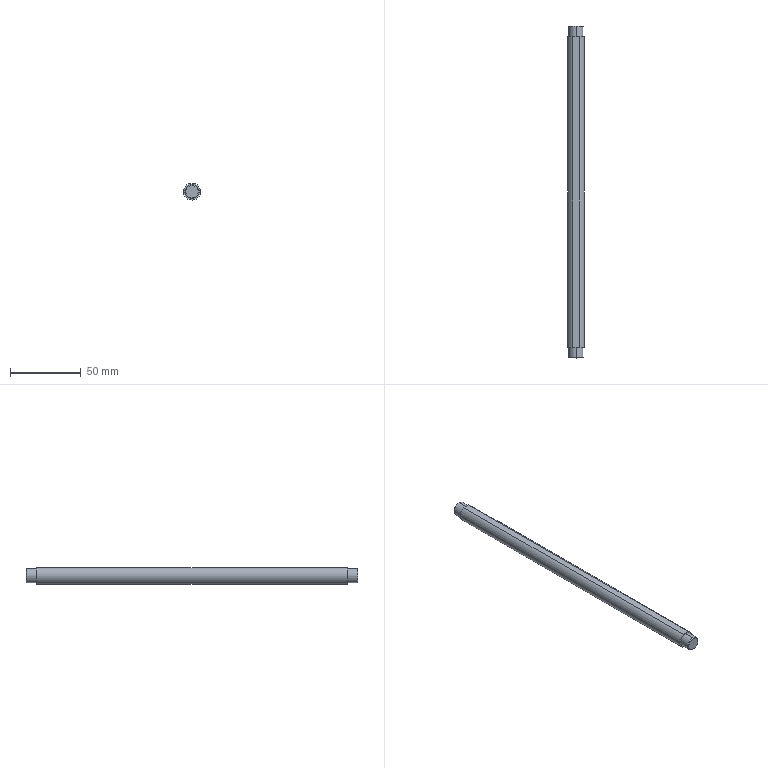Part | NX | features BREP 1 | 1 solid | 15 faces | box 12 x 235.2 x 11.5 mm | volume 25713 mm3 | cylinder 6 | plane 5 | cone 4 | commonest cylinder face diameters 10 x4 12 x2
STEP:
#1=CARTESIAN_POINT('',(0.,-117.1,-5.));
#2=VERTEX_POINT('',#1);
#3=CARTESIAN_POINT('',(0.,-117.6,-4.5));
#4=VERTEX_POINT('',#3);
#5=CARTESIAN_POINT('',(0.,-117.6,-4.5));
#6=DIRECTION('',(0.,0.7071,-0.7071));
#7=VECTOR('',#6,1000.);
#8=LINE('',#5,#7);
#9=EDGE_CURVE('',#2,#4,#8,.F.);
#10=ORIENTED_EDGE('',*,*,#9,.T.);
#11=CARTESIAN_POINT('',(0.,-117.6,4.5));
#12=VERTEX_POINT('',#11);
#13=CARTESIAN_POINT('',(0.,-117.6,0.));
#14=DIRECTION('',(0.,-1.,0.));
#15=DIRECTION('',(0.,0.,1.));
#16=AXIS2_PLACEMENT_3D('',#13,#14,#15);
#17=CIRCLE('',#16,4.5);
#18=EDGE_CURVE('',#12,#4,#17,.T.);
#19=ORIENTED_EDGE('',*,*,#18,.F.);
#20=CARTESIAN_POINT('',(0.,-117.1,5.));
#21=VERTEX_POINT('',#20);
#22=CARTESIAN_POINT('',(0.,-117.6,4.5));
#23=DIRECTION('',(0.,0.7071,0.7071));
#24=VECTOR('',#23,1000.);
#25=LINE('',#22,#24);
#26=EDGE_CURVE('',#21,#12,#25,.F.);
#27=ORIENTED_EDGE('',*,*,#26,.F.);
#28=CARTESIAN_POINT('',(0.,-117.1,0.));
#29=DIRECTION('',(0.,1.,0.));
#30=DIRECTION('',(0.,0.,1.));
#31=AXIS2_PLACEMENT_3D('',#28,#29,#30);
#32=CIRCLE('',#31,5.);
#33=EDGE_CURVE('',#2,#21,#32,.T.);
#34=ORIENTED_EDGE('',*,*,#33,.F.);
#35=EDGE_LOOP('',(#10,#19,#27,#34));
#36=FACE_BOUND('',#35,.T.);
#37=CARTESIAN_POINT('',(0.,-117.6,0.));
#38=DIRECTION('',(0.,1.,0.));
#39=DIRECTION('',(0.,0.,1.));
#40=AXIS2_PLACEMENT_3D('',#37,#38,#39);
#41=CONICAL_SURFACE('',#40,4.5,0.7854);
#42=ADVANCED_FACE('',(#36),#41,.T.);
#43=CARTESIAN_POINT('',(0.,117.6,4.5));
#44=VERTEX_POINT('',#43);
#45=CARTESIAN_POINT('',(0.,117.1,5.));
#46=VERTEX_POINT('',#45);
#47=CARTESIAN_POINT('',(0.,117.1,5.));
#48=DIRECTION('',(0.,-0.7071,0.7071));
#49=VECTOR('',#48,1000.);
#50=LINE('',#47,#49);
#51=EDGE_CURVE('',#44,#46,#50,.T.);
#52=ORIENTED_EDGE('',*,*,#51,.F.);
#53=CARTESIAN_POINT('',(0.,117.6,-4.5));
#54=VERTEX_POINT('',#53);
#55=CARTESIAN_POINT('',(0.,117.6,0.));
#56=DIRECTION('',(0.,1.,0.));
#57=DIRECTION('',(0.,0.,-1.));
#58=AXIS2_PLACEMENT_3D('',#55,#56,#57);
#59=CIRCLE('',#58,4.5);
#60=EDGE_CURVE('',#54,#44,#59,.T.);
#61=ORIENTED_EDGE('',*,*,#60,.F.);
#62=CARTESIAN_POINT('',(0.,117.1,-5.));
#63=VERTEX_POINT('',#62);
#64=CARTESIAN_POINT('',(0.,117.1,-5.));
#65=DIRECTION('',(0.,-0.7071,-0.7071));
#66=VECTOR('',#65,1000.);
#67=LINE('',#64,#66);
#68=EDGE_CURVE('',#54,#63,#67,.T.);
#69=ORIENTED_EDGE('',*,*,#68,.T.);
#70=CARTESIAN_POINT('',(0.,117.1,0.));
#71=DIRECTION('',(0.,-1.,0.));
#72=DIRECTION('',(0.,0.,-1.));
#73=AXIS2_PLACEMENT_3D('',#70,#71,#72);
#74=CIRCLE('',#73,5.);
#75=EDGE_CURVE('',#46,#63,#74,.T.);
#76=ORIENTED_EDGE('',*,*,#75,.F.);
#77=EDGE_LOOP('',(#52,#61,#69,#76));
#78=FACE_BOUND('',#77,.T.);
#79=CARTESIAN_POINT('',(0.,117.1,0.));
#80=DIRECTION('',(0.,-1.,0.));
#81=DIRECTION('',(0.,0.,-1.));
#82=AXIS2_PLACEMENT_3D('',#79,#80,#81);
#83=CONICAL_SURFACE('',#82,5.,0.7854);
#84=ADVANCED_FACE('',(#78),#83,.T.);
#85=CARTESIAN_POINT('',(2.398,-110.,5.5));
#86=VERTEX_POINT('',#85);
#87=CARTESIAN_POINT('',(2.398,110.,5.5));
#88=VERTEX_POINT('',#87);
#89=CARTESIAN_POINT('',(2.398,-117.6,5.5));
#90=DIRECTION('',(0.,1.,0.));
#91=VECTOR('',#90,1000.);
#92=LINE('',#89,#91);
#93=EDGE_CURVE('',#86,#88,#92,.T.);
#94=ORIENTED_EDGE('',*,*,#93,.T.);
#95=CARTESIAN_POINT('',(-2.398,110.,5.5));
#96=VERTEX_POINT('',#95);
#97=CARTESIAN_POINT('',(2.398,110.,5.5));
#98=DIRECTION('',(-1.,0.,0.));
#99=VECTOR('',#98,1000.);
#100=LINE('',#97,#99);
#101=EDGE_CURVE('',#88,#96,#100,.T.);
#102=ORIENTED_EDGE('',*,*,#101,.T.);
#103=CARTESIAN_POINT('',(-2.398,-110.,5.5));
#104=VERTEX_POINT('',#103);
#105=CARTESIAN_POINT('',(-2.398,-117.6,5.5));
#106=DIRECTION('',(0.,1.,0.));
#107=VECTOR('',#106,1000.);
#108=LINE('',#105,#107);
#109=EDGE_CURVE('',#104,#96,#108,.T.);
#110=ORIENTED_EDGE('',*,*,#109,.F.);
#111=CARTESIAN_POINT('',(-5.,-110.,5.5));
#112=DIRECTION('',(-1.,0.,0.));
#113=VECTOR('',#112,1000.);
#114=LINE('',#111,#113);
#115=EDGE_CURVE('',#86,#104,#114,.T.);
#116=ORIENTED_EDGE('',*,*,#115,.F.);
#117=EDGE_LOOP('',(#94,#102,#110,#116));
#118=FACE_BOUND('',#117,.T.);
#119=CARTESIAN_POINT('',(2.398,-117.6,5.5));
#120=DIRECTION('',(0.,0.,-1.));
#121=DIRECTION('',(-1.,0.,0.));
#122=AXIS2_PLACEMENT_3D('',#119,#120,#121);
#123=PLANE('',#122);
#124=ADVANCED_FACE('',(#118),#123,.F.);
#125=ORIENTED_EDGE('',*,*,#18,.T.);
#126=CARTESIAN_POINT('',(0.,-117.6,0.));
#127=DIRECTION('',(0.,-1.,0.));
#128=DIRECTION('',(0.,0.,1.));
#129=AXIS2_PLACEMENT_3D('',#126,#127,#128);
#130=CIRCLE('',#129,4.5);
#131=EDGE_CURVE('',#4,#12,#130,.T.);
#132=ORIENTED_EDGE('',*,*,#131,.T.);
#133=EDGE_LOOP('',(#125,#132));
#134=FACE_BOUND('',#133,.T.);
#135=CARTESIAN_POINT('',(-5.,-117.6,0.));
#136=DIRECTION('',(0.,1.,0.));
#137=DIRECTION('',(0.,0.,1.));
#138=AXIS2_PLACEMENT_3D('',#135,#136,#137);
#139=PLANE('',#138);
#140=ADVANCED_FACE('',(#134),#139,.F.);
#141=CARTESIAN_POINT('',(0.,-110.,5.));
#142=VERTEX_POINT('',#141);
#143=CARTESIAN_POINT('',(0.,0.,5.));
#144=DIRECTION('',(0.,-1.,0.));
#145=VECTOR('',#144,1000.);
#146=LINE('',#143,#145);
#147=EDGE_CURVE('',#142,#21,#146,.T.);
#148=ORIENTED_EDGE('',*,*,#147,.F.);
#149=CARTESIAN_POINT('',(0.,-110.,-5.));
#150=VERTEX_POINT('',#149);
#151=CARTESIAN_POINT('',(0.,-110.,0.));
#152=DIRECTION('',(0.,-1.,0.));
#153=DIRECTION('',(0.,0.,-1.));
#154=AXIS2_PLACEMENT_3D('',#151,#152,#153);
#155=CIRCLE('',#154,5.);
#156=EDGE_CURVE('',#142,#150,#155,.T.);
#157=ORIENTED_EDGE('',*,*,#156,.T.);
#158=CARTESIAN_POINT('',(0.,0.,-5.));
#159=DIRECTION('',(0.,-1.,0.));
#160=VECTOR('',#159,1000.);
#161=LINE('',#158,#160);
#162=EDGE_CURVE('',#150,#2,#161,.T.);
#163=ORIENTED_EDGE('',*,*,#162,.T.);
#164=ORIENTED_EDGE('',*,*,#33,.T.);
#165=EDGE_LOOP('',(#148,#157,#163,#164));
#166=FACE_BOUND('',#165,.T.);
#167=CARTESIAN_POINT('',(0.,0.,0.));
#168=DIRECTION('',(0.,-1.,0.));
#169=DIRECTION('',(0.,0.,-1.));
#170=AXIS2_PLACEMENT_3D('',#167,#168,#169);
#171=CYLINDRICAL_SURFACE('',#170,5.);
#172=ADVANCED_FACE('',(#166),#171,.T.);
#173=CARTESIAN_POINT('',(0.,-110.,-6.));
#174=VERTEX_POINT('',#173);
#175=CARTESIAN_POINT('',(0.,-110.,0.));
#176=DIRECTION('',(0.,-1.,0.));
#177=DIRECTION('',(0.,0.,-1.));
#178=AXIS2_PLACEMENT_3D('',#175,#176,#177);
#179=CIRCLE('',#178,6.);
#180=EDGE_CURVE('',#104,#174,#179,.T.);
#181=ORIENTED_EDGE('',*,*,#180,.T.);
#182=CARTESIAN_POINT('',(0.,-110.,0.));
#183=DIRECTION('',(0.,-1.,0.));
#184=DIRECTION('',(0.,0.,-1.));
#185=AXIS2_PLACEMENT_3D('',#182,#183,#184);
#186=CIRCLE('',#185,6.);
#187=EDGE_CURVE('',#174,#86,#186,.T.);
#188=ORIENTED_EDGE('',*,*,#187,.T.);
#189=ORIENTED_EDGE('',*,*,#115,.T.);
#190=EDGE_LOOP('',(#181,#188,#189));
#191=FACE_BOUND('',#190,.T.);
#192=CARTESIAN_POINT('',(0.,-110.,0.));
#193=DIRECTION('',(0.,-1.,0.));
#194=DIRECTION('',(0.,0.,-1.));
#195=AXIS2_PLACEMENT_3D('',#192,#193,#194);
#196=CIRCLE('',#195,5.);
#197=EDGE_CURVE('',#150,#142,#196,.T.);
#198=ORIENTED_EDGE('',*,*,#197,.F.);
#199=ORIENTED_EDGE('',*,*,#156,.F.);
#200=EDGE_LOOP('',(#198,#199));
#201=FACE_BOUND('',#200,.T.);
#202=CARTESIAN_POINT('',(-5.,-110.,0.));
#203=DIRECTION('',(0.,1.,0.));
#204=DIRECTION('',(0.,0.,1.));
#205=AXIS2_PLACEMENT_3D('',#202,#203,#204);
#206=PLANE('',#205);
#207=ADVANCED_FACE('',(#191,#201),#206,.F.);
#208=CARTESIAN_POINT('',(0.,110.,-6.));
#209=VERTEX_POINT('',#208);
#210=CARTESIAN_POINT('',(0.,0.,-6.));
#211=DIRECTION('',(0.,-1.,0.));
#212=VECTOR('',#211,1000.);
#213=LINE('',#210,#212);
#214=EDGE_CURVE('',#209,#174,#213,.T.);
#215=ORIENTED_EDGE('',*,*,#214,.F.);
#216=CARTESIAN_POINT('',(0.,110.,0.));
#217=DIRECTION('',(0.,-1.,0.));
#218=DIRECTION('',(0.,0.,-1.));
#219=AXIS2_PLACEMENT_3D('',#216,#217,#218);
#220=CIRCLE('',#219,6.);
#221=EDGE_CURVE('',#209,#88,#220,.T.);
#222=ORIENTED_EDGE('',*,*,#221,.T.);
#223=ORIENTED_EDGE('',*,*,#93,.F.);
#224=ORIENTED_EDGE('',*,*,#187,.F.);
#225=EDGE_LOOP('',(#215,#222,#223,#224));
#226=FACE_BOUND('',#225,.T.);
#227=CARTESIAN_POINT('',(0.,0.,0.));
#228=DIRECTION('',(0.,-1.,0.));
#229=DIRECTION('',(0.,0.,-1.));
#230=AXIS2_PLACEMENT_3D('',#227,#228,#229);
#231=CYLINDRICAL_SURFACE('',#230,6.);
#232=ADVANCED_FACE('',(#226),#231,.T.);
#233=CARTESIAN_POINT('',(0.,110.,-5.));
#234=VERTEX_POINT('',#233);
#235=CARTESIAN_POINT('',(0.,110.,5.));
#236=VERTEX_POINT('',#235);
#237=CARTESIAN_POINT('',(0.,110.,0.));
#238=DIRECTION('',(0.,-1.,0.));
#239=DIRECTION('',(0.,0.,-1.));
#240=AXIS2_PLACEMENT_3D('',#237,#238,#239);
#241=CIRCLE('',#240,5.);
#242=EDGE_CURVE('',#234,#236,#241,.T.);
#243=ORIENTED_EDGE('',*,*,#242,.T.);
#244=CARTESIAN_POINT('',(0.,110.,0.));
#245=DIRECTION('',(0.,-1.,0.));
#246=DIRECTION('',(0.,0.,-1.));
#247=AXIS2_PLACEMENT_3D('',#244,#245,#246);
#248=CIRCLE('',#247,5.);
#249=EDGE_CURVE('',#236,#234,#248,.T.);
#250=ORIENTED_EDGE('',*,*,#249,.T.);
#251=EDGE_LOOP('',(#243,#250));
#252=FACE_BOUND('',#251,.T.);
#253=CARTESIAN_POINT('',(0.,110.,0.));
#254=DIRECTION('',(0.,-1.,0.));
#255=DIRECTION('',(0.,0.,-1.));
#256=AXIS2_PLACEMENT_3D('',#253,#254,#255);
#257=CIRCLE('',#256,6.);
#258=EDGE_CURVE('',#96,#209,#257,.T.);
#259=ORIENTED_EDGE('',*,*,#258,.F.);
#260=ORIENTED_EDGE('',*,*,#101,.F.);
#261=ORIENTED_EDGE('',*,*,#221,.F.);
#262=EDGE_LOOP('',(#259,#260,#261));
#263=FACE_BOUND('',#262,.T.);
#264=CARTESIAN_POINT('',(-5.,110.,0.));
#265=DIRECTION('',(0.,-1.,0.));
#266=DIRECTION('',(0.,0.,-1.));
#267=AXIS2_PLACEMENT_3D('',#264,#265,#266);
#268=PLANE('',#267);
#269=ADVANCED_FACE('',(#252,#263),#268,.F.);
#270=CARTESIAN_POINT('',(0.,0.,5.));
#271=DIRECTION('',(0.,-1.,0.));
#272=VECTOR('',#271,1000.);
#273=LINE('',#270,#272);
#274=EDGE_CURVE('',#46,#236,#273,.T.);
#275=ORIENTED_EDGE('',*,*,#274,.F.);
#276=ORIENTED_EDGE('',*,*,#75,.T.);
#277=CARTESIAN_POINT('',(0.,0.,-5.));
#278=DIRECTION('',(0.,-1.,0.));
#279=VECTOR('',#278,1000.);
#280=LINE('',#277,#279);
#281=EDGE_CURVE('',#63,#234,#280,.T.);
#282=ORIENTED_EDGE('',*,*,#281,.T.);
#283=ORIENTED_EDGE('',*,*,#249,.F.);
#284=EDGE_LOOP('',(#275,#276,#282,#283));
#285=FACE_BOUND('',#284,.T.);
#286=CARTESIAN_POINT('',(0.,0.,0.));
#287=DIRECTION('',(0.,-1.,0.));
#288=DIRECTION('',(0.,0.,-1.));
#289=AXIS2_PLACEMENT_3D('',#286,#287,#288);
#290=CYLINDRICAL_SURFACE('',#289,5.);
#291=ADVANCED_FACE('',(#285),#290,.T.);
#292=ORIENTED_EDGE('',*,*,#60,.T.);
#293=CARTESIAN_POINT('',(0.,117.6,0.));
#294=DIRECTION('',(0.,1.,0.));
#295=DIRECTION('',(0.,0.,-1.));
#296=AXIS2_PLACEMENT_3D('',#293,#294,#295);
#297=CIRCLE('',#296,4.5);
#298=EDGE_CURVE('',#44,#54,#297,.T.);
#299=ORIENTED_EDGE('',*,*,#298,.T.);
#300=EDGE_LOOP('',(#292,#299));
#301=FACE_BOUND('',#300,.T.);
#302=CARTESIAN_POINT('',(-5.,117.6,0.));
#303=DIRECTION('',(0.,-1.,0.));
#304=DIRECTION('',(0.,0.,-1.));
#305=AXIS2_PLACEMENT_3D('',#302,#303,#304);
#306=PLANE('',#305);
#307=ADVANCED_FACE('',(#301),#306,.F.);
#308=CARTESIAN_POINT('',(0.,117.1,0.));
#309=DIRECTION('',(0.,-1.,0.));
#310=DIRECTION('',(0.,0.,-1.));
#311=AXIS2_PLACEMENT_3D('',#308,#309,#310);
#312=CIRCLE('',#311,5.);
#313=EDGE_CURVE('',#63,#46,#312,.T.);
#314=ORIENTED_EDGE('',*,*,#313,.T.);
#315=ORIENTED_EDGE('',*,*,#274,.T.);
#316=ORIENTED_EDGE('',*,*,#242,.F.);
#317=ORIENTED_EDGE('',*,*,#281,.F.);
#318=EDGE_LOOP('',(#314,#315,#316,#317));
#319=FACE_BOUND('',#318,.T.);
#320=CARTESIAN_POINT('',(0.,0.,0.));
#321=DIRECTION('',(0.,-1.,0.));
#322=DIRECTION('',(0.,0.,-1.));
#323=AXIS2_PLACEMENT_3D('',#320,#321,#322);
#324=CYLINDRICAL_SURFACE('',#323,5.);
#325=ADVANCED_FACE('',(#319),#324,.T.);
#326=ORIENTED_EDGE('',*,*,#258,.T.);
#327=ORIENTED_EDGE('',*,*,#214,.T.);
#328=ORIENTED_EDGE('',*,*,#180,.F.);
#329=ORIENTED_EDGE('',*,*,#109,.T.);
#330=EDGE_LOOP('',(#326,#327,#328,#329));
#331=FACE_BOUND('',#330,.T.);
#332=CARTESIAN_POINT('',(0.,0.,0.));
#333=DIRECTION('',(0.,-1.,0.));
#334=DIRECTION('',(0.,0.,-1.));
#335=AXIS2_PLACEMENT_3D('',#332,#333,#334);
#336=CYLINDRICAL_SURFACE('',#335,6.);
#337=ADVANCED_FACE('',(#331),#336,.T.);
#338=ORIENTED_EDGE('',*,*,#197,.T.);
#339=ORIENTED_EDGE('',*,*,#147,.T.);
#340=CARTESIAN_POINT('',(0.,-117.1,0.));
#341=DIRECTION('',(0.,1.,0.));
#342=DIRECTION('',(0.,0.,1.));
#343=AXIS2_PLACEMENT_3D('',#340,#341,#342);
#344=CIRCLE('',#343,5.);
#345=EDGE_CURVE('',#21,#2,#344,.T.);
#346=ORIENTED_EDGE('',*,*,#345,.T.);
#347=ORIENTED_EDGE('',*,*,#162,.F.);
#348=EDGE_LOOP('',(#338,#339,#346,#347));
#349=FACE_BOUND('',#348,.T.);
#350=CARTESIAN_POINT('',(0.,0.,0.));
#351=DIRECTION('',(0.,-1.,0.));
#352=DIRECTION('',(0.,0.,-1.));
#353=AXIS2_PLACEMENT_3D('',#350,#351,#352);
#354=CYLINDRICAL_SURFACE('',#353,5.);
#355=ADVANCED_FACE('',(#349),#354,.T.);
#356=ORIENTED_EDGE('',*,*,#298,.F.);
#357=ORIENTED_EDGE('',*,*,#51,.T.);
#358=ORIENTED_EDGE('',*,*,#313,.F.);
#359=ORIENTED_EDGE('',*,*,#68,.F.);
#360=EDGE_LOOP('',(#356,#357,#358,#359));
#361=FACE_BOUND('',#360,.T.);
#362=CARTESIAN_POINT('',(0.,117.1,0.));
#363=DIRECTION('',(0.,-1.,0.));
#364=DIRECTION('',(0.,0.,-1.));
#365=AXIS2_PLACEMENT_3D('',#362,#363,#364);
#366=CONICAL_SURFACE('',#365,5.,0.7854);
#367=ADVANCED_FACE('',(#361),#366,.T.);
#368=ORIENTED_EDGE('',*,*,#131,.F.);
#369=ORIENTED_EDGE('',*,*,#9,.F.);
#370=ORIENTED_EDGE('',*,*,#345,.F.);
#371=ORIENTED_EDGE('',*,*,#26,.T.);
#372=EDGE_LOOP('',(#368,#369,#370,#371));
#373=FACE_BOUND('',#372,.T.);
#374=CARTESIAN_POINT('',(0.,-117.6,0.));
#375=DIRECTION('',(0.,1.,0.));
#376=DIRECTION('',(0.,0.,1.));
#377=AXIS2_PLACEMENT_3D('',#374,#375,#376);
#378=CONICAL_SURFACE('',#377,4.5,0.7854);
#379=ADVANCED_FACE('',(#373),#378,.T.);
#380=CLOSED_SHELL('',(#42,#84,#124,#140,#172,#207,#232,#269,#291,#307,#325,#337,#355,#367,#379));
#381=MANIFOLD_SOLID_BREP('',#380);
#382=(LENGTH_UNIT()NAMED_UNIT(*)SI_UNIT(.MILLI.,.METRE.));
#383=UNCERTAINTY_MEASURE_WITH_UNIT(LENGTH_MEASURE(0.00001),#382,'','');
#384=(NAMED_UNIT(*)PLANE_ANGLE_UNIT()SI_UNIT($,.RADIAN.));
#385=(NAMED_UNIT(*)SI_UNIT($,.STERADIAN.)SOLID_ANGLE_UNIT());
#386=(GEOMETRIC_REPRESENTATION_CONTEXT(3)GLOBAL_UNCERTAINTY_ASSIGNED_CONTEXT((#383))GLOBAL_UNIT_ASSIGNED_CONTEXT((#382,#384,#385))REPRESENTATION_CONTEXT('',''));
#387=ADVANCED_BREP_SHAPE_REPRESENTATION('',(#381),#386);